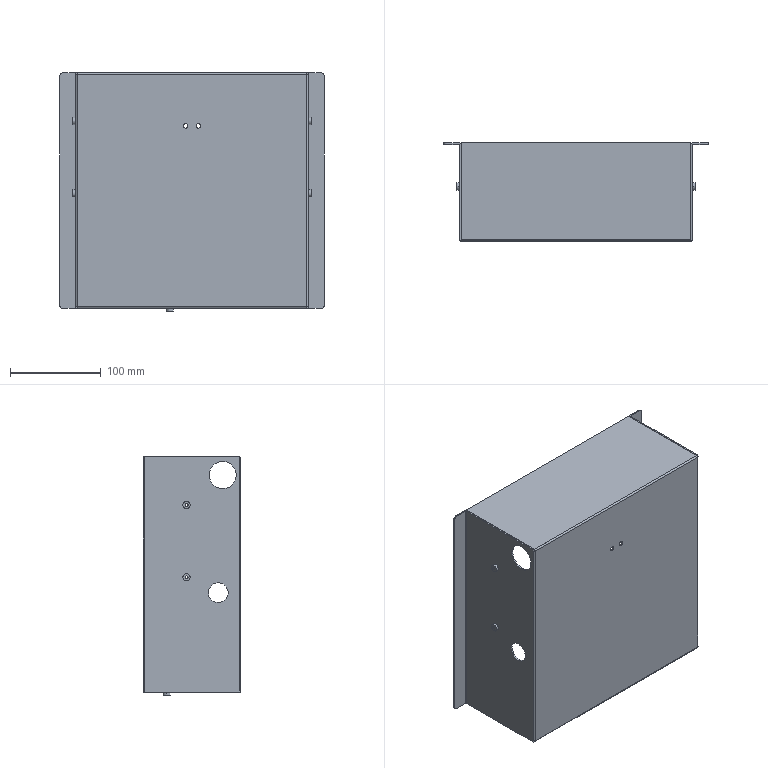Part | SolidWorks | features ICE 9, MirrorPattern 3, EdgeFlange 2, 3DProfileFeature 1, Fillet 1, FlatPattern 1, HoleWzd 1, SMBaseFlange 1, SheetMetal 1 | 1 solid | 117 faces | box 292 x 108 x 263 mm | volume 272152 mm3 | plane 59 | cylinder 58 | commonest cylinder face diameters 3.2 x10 6 x10 8 x10 0.4 x6 3.4 x6 5 x4